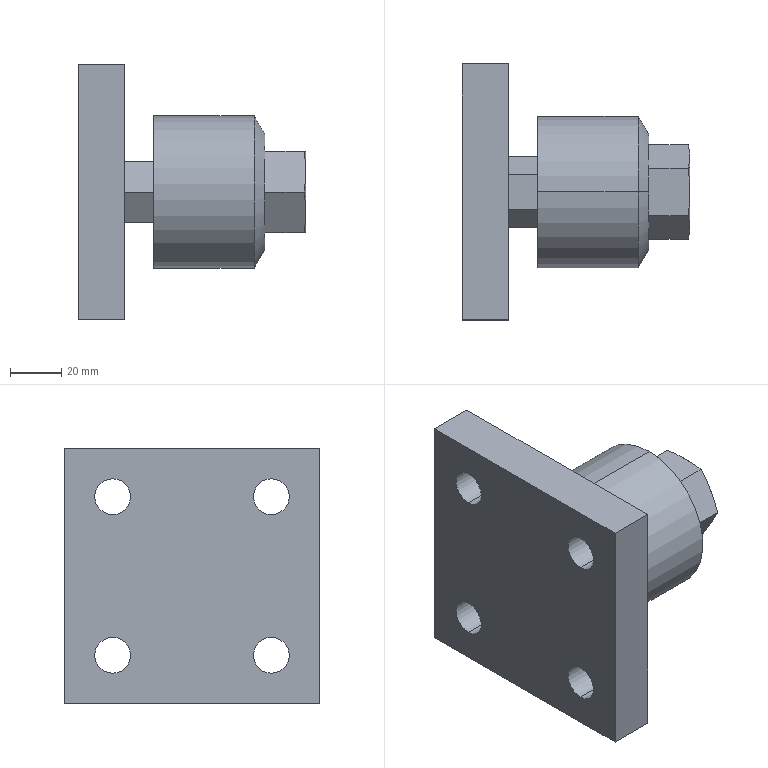Part | SolidWorks | features BaseBody 2 | 2 solids | 46 faces | box 89 x 100 x 100 mm | volume 301909 mm3 | plane 22 | cylinder 12 | cone 12 | commonest cylinder face diameters 14 x8 18.376 x2 59.5 x2
STEP:
#1=CARTESIAN_POINT('',(-59.5,0.,-29.75));
#2=VERTEX_POINT('',#1);
#3=CARTESIAN_POINT('',(-59.5,0.,29.75));
#4=VERTEX_POINT('',#3);
#5=CARTESIAN_POINT('',(-59.5,0.,0.));
#6=DIRECTION('',(1.,0.,0.));
#7=DIRECTION('',(0.,0.,-1.));
#8=AXIS2_PLACEMENT_3D('',#5,#6,#7);
#9=CIRCLE('',#8,29.75);
#10=EDGE_CURVE('',#2,#4,#9,.T.);
#11=ORIENTED_EDGE('',*,*,#10,.T.);
#12=CARTESIAN_POINT('',(-20.186,0.,29.75));
#13=VERTEX_POINT('',#12);
#14=CARTESIAN_POINT('',(-39.843,0.,29.75));
#15=DIRECTION('',(1.,0.,0.));
#16=VECTOR('',#15,1000.);
#17=LINE('',#14,#16);
#18=EDGE_CURVE('',#4,#13,#17,.T.);
#19=ORIENTED_EDGE('',*,*,#18,.T.);
#20=CARTESIAN_POINT('',(-20.186,0.,-29.75));
#21=VERTEX_POINT('',#20);
#22=CARTESIAN_POINT('',(-20.186,0.,0.));
#23=DIRECTION('',(-1.,0.,0.));
#24=DIRECTION('',(0.,0.,-1.));
#25=AXIS2_PLACEMENT_3D('',#22,#23,#24);
#26=CIRCLE('',#25,29.75);
#27=EDGE_CURVE('',#13,#21,#26,.T.);
#28=ORIENTED_EDGE('',*,*,#27,.T.);
#29=CARTESIAN_POINT('',(-39.843,0.,-29.75));
#30=DIRECTION('',(1.,0.,0.));
#31=VECTOR('',#30,1000.);
#32=LINE('',#29,#31);
#33=EDGE_CURVE('',#2,#21,#32,.T.);
#34=ORIENTED_EDGE('',*,*,#33,.F.);
#35=EDGE_LOOP('',(#11,#19,#28,#34));
#36=FACE_OUTER_BOUND('',#35,.T.);
#37=CARTESIAN_POINT('',(-39.843,0.,0.));
#38=DIRECTION('',(1.,0.,0.));
#39=DIRECTION('',(0.,0.,-1.));
#40=AXIS2_PLACEMENT_3D('',#37,#38,#39);
#41=CYLINDRICAL_SURFACE('',#40,29.75);
#42=ADVANCED_FACE('',(#36),#41,.T.);
#43=CARTESIAN_POINT('',(-16.,0.,22.5));
#44=VERTEX_POINT('',#43);
#45=CARTESIAN_POINT('',(-16.,0.,-22.5));
#46=VERTEX_POINT('',#45);
#47=CARTESIAN_POINT('',(-16.,0.,0.));
#48=DIRECTION('',(-1.,0.,0.));
#49=DIRECTION('',(0.,0.,1.));
#50=AXIS2_PLACEMENT_3D('',#47,#48,#49);
#51=CIRCLE('',#50,22.5);
#52=EDGE_CURVE('',#44,#46,#51,.T.);
#53=ORIENTED_EDGE('',*,*,#52,.T.);
#54=CARTESIAN_POINT('',(-20.186,0.,-29.75));
#55=DIRECTION('',(-0.5,0.,-0.866));
#56=VECTOR('',#55,1000.);
#57=LINE('',#54,#56);
#58=EDGE_CURVE('',#46,#21,#57,.T.);
#59=ORIENTED_EDGE('',*,*,#58,.T.);
#60=ORIENTED_EDGE('',*,*,#27,.F.);
#61=CARTESIAN_POINT('',(-20.186,0.,29.75));
#62=DIRECTION('',(-0.5,0.,0.866));
#63=VECTOR('',#62,1000.);
#64=LINE('',#61,#63);
#65=EDGE_CURVE('',#44,#13,#64,.T.);
#66=ORIENTED_EDGE('',*,*,#65,.F.);
#67=EDGE_LOOP('',(#53,#59,#60,#66));
#68=FACE_OUTER_BOUND('',#67,.T.);
#69=CARTESIAN_POINT('',(-20.186,0.,0.));
#70=DIRECTION('',(-1.,0.,0.));
#71=DIRECTION('',(0.,0.,1.));
#72=AXIS2_PLACEMENT_3D('',#69,#70,#71);
#73=CONICAL_SURFACE('',#72,29.75,1.047);
#74=ADVANCED_FACE('',(#68),#73,.T.);
#75=CARTESIAN_POINT('',(-0.812,0.,9.188));
#76=VERTEX_POINT('',#75);
#77=CARTESIAN_POINT('',(-0.812,0.,-9.188));
#78=VERTEX_POINT('',#77);
#79=CARTESIAN_POINT('',(-0.812,0.,0.));
#80=DIRECTION('',(1.,0.,0.));
#81=DIRECTION('',(0.,0.,-1.));
#82=AXIS2_PLACEMENT_3D('',#79,#80,#81);
#83=CIRCLE('',#82,9.188);
#84=EDGE_CURVE('',#76,#78,#83,.T.);
#85=ORIENTED_EDGE('',*,*,#84,.F.);
#86=CARTESIAN_POINT('',(0.,0.,10.));
#87=VERTEX_POINT('',#86);
#88=CARTESIAN_POINT('',(0.,0.,10.));
#89=DIRECTION('',(0.7071,0.,0.7071));
#90=VECTOR('',#89,1000.);
#91=LINE('',#88,#90);
#92=EDGE_CURVE('',#76,#87,#91,.T.);
#93=ORIENTED_EDGE('',*,*,#92,.T.);
#94=CARTESIAN_POINT('',(0.,0.,-10.));
#95=VERTEX_POINT('',#94);
#96=CARTESIAN_POINT('',(0.,0.,0.));
#97=DIRECTION('',(-1.,0.,0.));
#98=DIRECTION('',(0.,0.,-1.));
#99=AXIS2_PLACEMENT_3D('',#96,#97,#98);
#100=CIRCLE('',#99,10.);
#101=EDGE_CURVE('',#95,#87,#100,.T.);
#102=ORIENTED_EDGE('',*,*,#101,.F.);
#103=CARTESIAN_POINT('',(0.,0.,-10.));
#104=DIRECTION('',(0.7071,0.,-0.7071));
#105=VECTOR('',#104,1000.);
#106=LINE('',#103,#105);
#107=EDGE_CURVE('',#78,#95,#106,.T.);
#108=ORIENTED_EDGE('',*,*,#107,.F.);
#109=EDGE_LOOP('',(#85,#93,#102,#108));
#110=FACE_OUTER_BOUND('',#109,.T.);
#111=CARTESIAN_POINT('',(0.,0.,0.));
#112=DIRECTION('',(1.,0.,0.));
#113=DIRECTION('',(0.,0.,-1.));
#114=AXIS2_PLACEMENT_3D('',#111,#112,#113);
#115=CONICAL_SURFACE('',#114,10.,0.7854);
#116=ADVANCED_FACE('',(#110),#115,.F.);
#117=CARTESIAN_POINT('',(-18.,0.,9.188));
#118=VERTEX_POINT('',#117);
#119=CARTESIAN_POINT('',(-18.,0.,-9.188));
#120=VERTEX_POINT('',#119);
#121=CARTESIAN_POINT('',(-18.,0.,0.));
#122=DIRECTION('',(1.,0.,0.));
#123=DIRECTION('',(0.,0.,-1.));
#124=AXIS2_PLACEMENT_3D('',#121,#122,#123);
#125=CIRCLE('',#124,9.188);
#126=EDGE_CURVE('',#118,#120,#125,.T.);
#127=ORIENTED_EDGE('',*,*,#126,.F.);
#128=CARTESIAN_POINT('',(-9.406,0.,9.188));
#129=DIRECTION('',(1.,0.,0.));
#130=VECTOR('',#129,1000.);
#131=LINE('',#128,#130);
#132=EDGE_CURVE('',#118,#76,#131,.T.);
#133=ORIENTED_EDGE('',*,*,#132,.T.);
#134=ORIENTED_EDGE('',*,*,#84,.T.);
#135=CARTESIAN_POINT('',(-9.406,0.,-9.188));
#136=DIRECTION('',(1.,0.,0.));
#137=VECTOR('',#136,1000.);
#138=LINE('',#135,#137);
#139=EDGE_CURVE('',#120,#78,#138,.T.);
#140=ORIENTED_EDGE('',*,*,#139,.F.);
#141=EDGE_LOOP('',(#127,#133,#134,#140));
#142=FACE_OUTER_BOUND('',#141,.T.);
#143=CARTESIAN_POINT('',(-9.406,0.,0.));
#144=DIRECTION('',(1.,0.,0.));
#145=DIRECTION('',(0.,0.,-1.));
#146=AXIS2_PLACEMENT_3D('',#143,#144,#145);
#147=CYLINDRICAL_SURFACE('',#146,9.188);
#148=ADVANCED_FACE('',(#142),#147,.F.);
#149=CARTESIAN_POINT('',(-23.305,0.,0.));
#150=VERTEX_POINT('',#149);
#151=CARTESIAN_POINT('',(-18.,0.,-9.188));
#152=DIRECTION('',(0.5,0.,-0.866));
#153=VECTOR('',#152,1000.);
#154=LINE('',#151,#153);
#155=EDGE_CURVE('',#150,#120,#154,.T.);
#156=ORIENTED_EDGE('',*,*,#155,.F.);
#157=CARTESIAN_POINT('',(-18.,0.,9.188));
#158=DIRECTION('',(0.5,0.,0.866));
#159=VECTOR('',#158,1000.);
#160=LINE('',#157,#159);
#161=EDGE_CURVE('',#150,#118,#160,.T.);
#162=ORIENTED_EDGE('',*,*,#161,.T.);
#163=ORIENTED_EDGE('',*,*,#126,.T.);
#164=EDGE_LOOP('',(#156,#162,#163));
#165=FACE_OUTER_BOUND('',#164,.T.);
#166=CARTESIAN_POINT('',(-18.,0.,0.));
#167=DIRECTION('',(1.,0.,0.));
#168=DIRECTION('',(0.,0.,-1.));
#169=AXIS2_PLACEMENT_3D('',#166,#167,#168);
#170=CONICAL_SURFACE('',#169,9.188,1.047);
#171=ADVANCED_FACE('',(#165),#170,.F.);
#172=ORIENTED_EDGE('',*,*,#18,.F.);
#173=CARTESIAN_POINT('',(-59.5,0.,0.));
#174=DIRECTION('',(1.,0.,0.));
#175=DIRECTION('',(0.,0.,-1.));
#176=AXIS2_PLACEMENT_3D('',#173,#174,#175);
#177=CIRCLE('',#176,29.75);
#178=EDGE_CURVE('',#4,#2,#177,.T.);
#179=ORIENTED_EDGE('',*,*,#178,.T.);
#180=ORIENTED_EDGE('',*,*,#33,.T.);
#181=CARTESIAN_POINT('',(-20.186,0.,0.));
#182=DIRECTION('',(-1.,0.,0.));
#183=DIRECTION('',(0.,0.,-1.));
#184=AXIS2_PLACEMENT_3D('',#181,#182,#183);
#185=CIRCLE('',#184,29.75);
#186=EDGE_CURVE('',#21,#13,#185,.T.);
#187=ORIENTED_EDGE('',*,*,#186,.T.);
#188=EDGE_LOOP('',(#172,#179,#180,#187));
#189=FACE_OUTER_BOUND('',#188,.T.);
#190=CARTESIAN_POINT('',(-39.843,0.,0.));
#191=DIRECTION('',(1.,0.,0.));
#192=DIRECTION('',(0.,0.,-1.));
#193=AXIS2_PLACEMENT_3D('',#190,#191,#192);
#194=CYLINDRICAL_SURFACE('',#193,29.75);
#195=ADVANCED_FACE('',(#189),#194,.T.);
#196=ORIENTED_EDGE('',*,*,#58,.F.);
#197=CARTESIAN_POINT('',(-16.,0.,0.));
#198=DIRECTION('',(-1.,0.,0.));
#199=DIRECTION('',(0.,0.,1.));
#200=AXIS2_PLACEMENT_3D('',#197,#198,#199);
#201=CIRCLE('',#200,22.5);
#202=EDGE_CURVE('',#46,#44,#201,.T.);
#203=ORIENTED_EDGE('',*,*,#202,.T.);
#204=ORIENTED_EDGE('',*,*,#65,.T.);
#205=ORIENTED_EDGE('',*,*,#186,.F.);
#206=EDGE_LOOP('',(#196,#203,#204,#205));
#207=FACE_OUTER_BOUND('',#206,.T.);
#208=CARTESIAN_POINT('',(-20.186,0.,0.));
#209=DIRECTION('',(-1.,0.,0.));
#210=DIRECTION('',(0.,0.,1.));
#211=AXIS2_PLACEMENT_3D('',#208,#209,#210);
#212=CONICAL_SURFACE('',#211,29.75,1.047);
#213=ADVANCED_FACE('',(#207),#212,.T.);
#214=CARTESIAN_POINT('',(-59.5,-13.856,0.));
#215=VERTEX_POINT('',#214);
#216=CARTESIAN_POINT('',(-59.5,-6.928,-12.));
#217=VERTEX_POINT('',#216);
#218=CARTESIAN_POINT('',(-59.5,-13.856,0.));
#219=DIRECTION('',(0.,0.5,-0.866));
#220=VECTOR('',#219,1000.);
#221=LINE('',#218,#220);
#222=EDGE_CURVE('',#215,#217,#221,.T.);
#223=ORIENTED_EDGE('',*,*,#222,.T.);
#224=CARTESIAN_POINT('',(-59.5,6.928,-12.));
#225=VERTEX_POINT('',#224);
#226=CARTESIAN_POINT('',(-59.5,22.075,-12.));
#227=DIRECTION('',(0.,1.,0.));
#228=VECTOR('',#227,1000.);
#229=LINE('',#226,#228);
#230=EDGE_CURVE('',#217,#225,#229,.T.);
#231=ORIENTED_EDGE('',*,*,#230,.T.);
#232=CARTESIAN_POINT('',(-59.5,13.856,0.));
#233=VERTEX_POINT('',#232);
#234=CARTESIAN_POINT('',(-59.5,6.928,-12.));
#235=DIRECTION('',(0.,0.5,0.866));
#236=VECTOR('',#235,1000.);
#237=LINE('',#234,#236);
#238=EDGE_CURVE('',#225,#233,#237,.T.);
#239=ORIENTED_EDGE('',*,*,#238,.T.);
#240=CARTESIAN_POINT('',(-59.5,6.928,12.));
#241=VERTEX_POINT('',#240);
#242=CARTESIAN_POINT('',(-59.5,13.856,0.));
#243=DIRECTION('',(0.,-0.5,0.866));
#244=VECTOR('',#243,1000.);
#245=LINE('',#242,#244);
#246=EDGE_CURVE('',#233,#241,#245,.T.);
#247=ORIENTED_EDGE('',*,*,#246,.T.);
#248=CARTESIAN_POINT('',(-59.5,-6.928,12.));
#249=VERTEX_POINT('',#248);
#250=CARTESIAN_POINT('',(-59.5,22.075,12.));
#251=DIRECTION('',(0.,-1.,0.));
#252=VECTOR('',#251,1000.);
#253=LINE('',#250,#252);
#254=EDGE_CURVE('',#241,#249,#253,.T.);
#255=ORIENTED_EDGE('',*,*,#254,.T.);
#256=CARTESIAN_POINT('',(-59.5,-6.928,12.));
#257=DIRECTION('',(0.,-0.5,-0.866));
#258=VECTOR('',#257,1000.);
#259=LINE('',#256,#258);
#260=EDGE_CURVE('',#249,#215,#259,.T.);
#261=ORIENTED_EDGE('',*,*,#260,.T.);
#262=EDGE_LOOP('',(#223,#231,#239,#247,#255,#261));
#263=FACE_BOUND('',#262,.T.);
#264=ORIENTED_EDGE('',*,*,#10,.F.);
#265=ORIENTED_EDGE('',*,*,#178,.F.);
#266=EDGE_LOOP('',(#264,#265));
#267=FACE_OUTER_BOUND('',#266,.T.);
#268=CARTESIAN_POINT('',(-59.5,22.075,0.));
#269=DIRECTION('',(-1.,0.,0.));
#270=DIRECTION('',(0.,0.,1.));
#271=AXIS2_PLACEMENT_3D('',#268,#269,#270);
#272=PLANE('',#271);
#273=ADVANCED_FACE('',(#263,#267),#272,.T.);
#274=CARTESIAN_POINT('',(-16.,-9.238,16.));
#275=VERTEX_POINT('',#274);
#276=CARTESIAN_POINT('',(-16.,9.238,16.));
#277=VERTEX_POINT('',#276);
#278=CARTESIAN_POINT('',(-16.,20.488,16.));
#279=DIRECTION('',(0.,1.,0.));
#280=VECTOR('',#279,1000.);
#281=LINE('',#278,#280);
#282=EDGE_CURVE('',#275,#277,#281,.T.);
#283=ORIENTED_EDGE('',*,*,#282,.T.);
#284=CARTESIAN_POINT('',(-16.,18.475,0.));
#285=VERTEX_POINT('',#284);
#286=CARTESIAN_POINT('',(-16.,9.238,16.));
#287=DIRECTION('',(0.,0.5,-0.866));
#288=VECTOR('',#287,1000.);
#289=LINE('',#286,#288);
#290=EDGE_CURVE('',#277,#285,#289,.T.);
#291=ORIENTED_EDGE('',*,*,#290,.T.);
#292=CARTESIAN_POINT('',(-16.,9.238,-16.));
#293=VERTEX_POINT('',#292);
#294=CARTESIAN_POINT('',(-16.,18.475,0.));
#295=DIRECTION('',(0.,-0.5,-0.866));
#296=VECTOR('',#295,1000.);
#297=LINE('',#294,#296);
#298=EDGE_CURVE('',#285,#293,#297,.T.);
#299=ORIENTED_EDGE('',*,*,#298,.T.);
#300=CARTESIAN_POINT('',(-16.,-9.238,-16.));
#301=VERTEX_POINT('',#300);
#302=CARTESIAN_POINT('',(-16.,20.488,-16.));
#303=DIRECTION('',(0.,-1.,0.));
#304=VECTOR('',#303,1000.);
#305=LINE('',#302,#304);
#306=EDGE_CURVE('',#293,#301,#305,.T.);
#307=ORIENTED_EDGE('',*,*,#306,.T.);
#308=CARTESIAN_POINT('',(-16.,-18.475,0.));
#309=VERTEX_POINT('',#308);
#310=CARTESIAN_POINT('',(-16.,-9.238,-16.));
#311=DIRECTION('',(0.,-0.5,0.866));
#312=VECTOR('',#311,1000.);
#313=LINE('',#310,#312);
#314=EDGE_CURVE('',#301,#309,#313,.T.);
#315=ORIENTED_EDGE('',*,*,#314,.T.);
#316=CARTESIAN_POINT('',(-16.,-18.475,0.));
#317=DIRECTION('',(0.,0.5,0.866));
#318=VECTOR('',#317,1000.);
#319=LINE('',#316,#318);
#320=EDGE_CURVE('',#309,#275,#319,.T.);
#321=ORIENTED_EDGE('',*,*,#320,.T.);
#322=EDGE_LOOP('',(#283,#291,#299,#307,#315,#321));
#323=FACE_BOUND('',#322,.T.);
#324=ORIENTED_EDGE('',*,*,#52,.F.);
#325=ORIENTED_EDGE('',*,*,#202,.F.);
#326=EDGE_LOOP('',(#324,#325));
#327=FACE_OUTER_BOUND('',#326,.T.);
#328=CARTESIAN_POINT('',(-16.,20.488,0.));
#329=DIRECTION('',(1.,0.,0.));
#330=DIRECTION('',(0.,0.,-1.));
#331=AXIS2_PLACEMENT_3D('',#328,#329,#330);
#332=PLANE('',#331);
#333=ADVANCED_FACE('',(#323,#327),#332,.T.);
#334=CARTESIAN_POINT('',(-71.,6.928,-12.));
#335=VERTEX_POINT('',#334);
#336=CARTESIAN_POINT('',(-71.,-6.928,-12.));
#337=VERTEX_POINT('',#336);
#338=CARTESIAN_POINT('',(-71.,-6.928,-12.));
#339=DIRECTION('',(0.,-1.,0.));
#340=VECTOR('',#339,1000.);
#341=LINE('',#338,#340);
#342=EDGE_CURVE('',#335,#337,#341,.T.);
#343=ORIENTED_EDGE('',*,*,#342,.F.);
#344=CARTESIAN_POINT('',(-71.,6.928,-12.));
#345=DIRECTION('',(-1.,0.,0.));
#346=VECTOR('',#345,1000.);
#347=LINE('',#344,#346);
#348=EDGE_CURVE('',#225,#335,#347,.T.);
#349=ORIENTED_EDGE('',*,*,#348,.F.);
#350=ORIENTED_EDGE('',*,*,#230,.F.);
#351=CARTESIAN_POINT('',(-71.,-6.928,-12.));
#352=DIRECTION('',(1.,0.,0.));
#353=VECTOR('',#352,1000.);
#354=LINE('',#351,#353);
#355=EDGE_CURVE('',#337,#217,#354,.T.);
#356=ORIENTED_EDGE('',*,*,#355,.F.);
#357=EDGE_LOOP('',(#343,#349,#350,#356));
#358=FACE_OUTER_BOUND('',#357,.T.);
#359=CARTESIAN_POINT('',(-71.,-6.928,-12.));
#360=DIRECTION('',(0.,0.,1.));
#361=DIRECTION('',(1.,0.,0.));
#362=AXIS2_PLACEMENT_3D('',#359,#360,#361);
#363=PLANE('',#362);
#364=ADVANCED_FACE('',(#358),#363,.F.);
#365=CARTESIAN_POINT('',(-71.,-13.856,0.));
#366=VERTEX_POINT('',#365);
#367=CARTESIAN_POINT('',(-71.,-13.856,0.));
#368=DIRECTION('',(0.,-0.5,0.866));
#369=VECTOR('',#368,1000.);
#370=LINE('',#367,#369);
#371=EDGE_CURVE('',#337,#366,#370,.T.);
#372=ORIENTED_EDGE('',*,*,#371,.F.);
#373=ORIENTED_EDGE('',*,*,#355,.T.);
#374=ORIENTED_EDGE('',*,*,#222,.F.);
#375=CARTESIAN_POINT('',(-71.,-13.856,0.));
#376=DIRECTION('',(1.,0.,0.));
#377=VECTOR('',#376,1000.);
#378=LINE('',#375,#377);
#379=EDGE_CURVE('',#366,#215,#378,.T.);
#380=ORIENTED_EDGE('',*,*,#379,.F.);
#381=EDGE_LOOP('',(#372,#373,#374,#380));
#382=FACE_OUTER_BOUND('',#381,.T.);
#383=CARTESIAN_POINT('',(-71.,-13.856,0.));
#384=DIRECTION('',(0.,0.866,0.5));
#385=DIRECTION('',(0.,-0.5,0.866));
#386=AXIS2_PLACEMENT_3D('',#383,#384,#385);
#387=PLANE('',#386);
#388=ADVANCED_FACE('',(#382),#387,.F.);
#389=CARTESIAN_POINT('',(-71.,-6.928,12.));
#390=VERTEX_POINT('',#389);
#391=CARTESIAN_POINT('',(-71.,-6.928,12.));
#392=DIRECTION('',(0.,0.5,0.866));
#393=VECTOR('',#392,1000.);
#394=LINE('',#391,#393);
#395=EDGE_CURVE('',#366,#390,#394,.T.);
#396=ORIENTED_EDGE('',*,*,#395,.F.);
#397=ORIENTED_EDGE('',*,*,#379,.T.);
#398=ORIENTED_EDGE('',*,*,#260,.F.);
#399=CARTESIAN_POINT('',(-71.,-6.928,12.));
#400=DIRECTION('',(1.,0.,0.));
#401=VECTOR('',#400,1000.);
#402=LINE('',#399,#401);
#403=EDGE_CURVE('',#390,#249,#402,.T.);
#404=ORIENTED_EDGE('',*,*,#403,.F.);
#405=EDGE_LOOP('',(#396,#397,#398,#404));
#406=FACE_OUTER_BOUND('',#405,.T.);
#407=CARTESIAN_POINT('',(-71.,-6.928,12.));
#408=DIRECTION('',(0.,0.866,-0.5));
#409=DIRECTION('',(0.,0.5,0.866));
#410=AXIS2_PLACEMENT_3D('',#407,#408,#409);
#411=PLANE('',#410);
#412=ADVANCED_FACE('',(#406),#411,.F.);
#413=CARTESIAN_POINT('',(-71.,6.928,12.));
#414=VERTEX_POINT('',#413);
#415=CARTESIAN_POINT('',(-71.,6.928,12.));
#416=DIRECTION('',(0.,1.,0.));
#417=VECTOR('',#416,1000.);
#418=LINE('',#415,#417);
#419=EDGE_CURVE('',#390,#414,#418,.T.);
#420=ORIENTED_EDGE('',*,*,#419,.F.);
#421=ORIENTED_EDGE('',*,*,#403,.T.);
#422=ORIENTED_EDGE('',*,*,#254,.F.);
#423=CARTESIAN_POINT('',(-71.,6.928,12.));
#424=DIRECTION('',(1.,0.,0.));
#425=VECTOR('',#424,1000.);
#426=LINE('',#423,#425);
#427=EDGE_CURVE('',#414,#241,#426,.T.);
#428=ORIENTED_EDGE('',*,*,#427,.F.);
#429=EDGE_LOOP('',(#420,#421,#422,#428));
#430=FACE_OUTER_BOUND('',#429,.T.);
#431=CARTESIAN_POINT('',(-71.,6.928,12.));
#432=DIRECTION('',(0.,0.,-1.));
#433=DIRECTION('',(-1.,0.,0.));
#434=AXIS2_PLACEMENT_3D('',#431,#432,#433);
#435=PLANE('',#434);
#436=ADVANCED_FACE('',(#430),#435,.F.);
#437=CARTESIAN_POINT('',(-71.,13.856,0.));
#438=VERTEX_POINT('',#437);
#439=CARTESIAN_POINT('',(-71.,13.856,0.));
#440=DIRECTION('',(0.,0.5,-0.866));
#441=VECTOR('',#440,1000.);
#442=LINE('',#439,#441);
#443=EDGE_CURVE('',#414,#438,#442,.T.);
#444=ORIENTED_EDGE('',*,*,#443,.F.);
#445=ORIENTED_EDGE('',*,*,#427,.T.);
#446=ORIENTED_EDGE('',*,*,#246,.F.);
#447=CARTESIAN_POINT('',(-71.,13.856,0.));
#448=DIRECTION('',(1.,0.,0.));
#449=VECTOR('',#448,1000.);
#450=LINE('',#447,#449);
#451=EDGE_CURVE('',#438,#233,#450,.T.);
#452=ORIENTED_EDGE('',*,*,#451,.F.);
#453=EDGE_LOOP('',(#444,#445,#446,#452));
#454=FACE_OUTER_BOUND('',#453,.T.);
#455=CARTESIAN_POINT('',(-71.,13.856,0.));
#456=DIRECTION('',(0.,-0.866,-0.5));
#457=DIRECTION('',(0.,0.5,-0.866));
#458=AXIS2_PLACEMENT_3D('',#455,#456,#457);
#459=PLANE('',#458);
#460=ADVANCED_FACE('',(#454),#459,.F.);
#461=CARTESIAN_POINT('',(-71.,6.928,-12.));
#462=DIRECTION('',(0.,-0.5,-0.866));
#463=VECTOR('',#462,1000.);
#464=LINE('',#461,#463);
#465=EDGE_CURVE('',#438,#335,#464,.T.);
#466=ORIENTED_EDGE('',*,*,#465,.F.);
#467=ORIENTED_EDGE('',*,*,#451,.T.);
#468=ORIENTED_EDGE('',*,*,#238,.F.);
#469=ORIENTED_EDGE('',*,*,#348,.T.);
#470=EDGE_LOOP('',(#466,#467,#468,#469));
#471=FACE_OUTER_BOUND('',#470,.T.);
#472=CARTESIAN_POINT('',(-71.,6.928,-12.));
#473=DIRECTION('',(0.,-0.866,0.5));
#474=DIRECTION('',(0.,-0.5,-0.866));
#475=AXIS2_PLACEMENT_3D('',#472,#473,#474);
#476=PLANE('',#475);
#477=ADVANCED_FACE('',(#471),#476,.F.);
#478=ORIENTED_EDGE('',*,*,#290,.F.);
#479=CARTESIAN_POINT('',(-0.6632,9.238,16.));
#480=VERTEX_POINT('',#479);
#481=CARTESIAN_POINT('',(0.,9.238,16.));
#482=DIRECTION('',(-1.,0.,0.));
#483=VECTOR('',#482,1000.);
#484=LINE('',#481,#483);
#485=EDGE_CURVE('',#480,#277,#484,.T.);
#486=ORIENTED_EDGE('',*,*,#485,.F.);
#487=CARTESIAN_POINT('',(0.,13.856,8.));
#488=VERTEX_POINT('',#487);
#489=CARTESIAN_POINT('',(0.,13.856,8.));
#490=CARTESIAN_POINT('',(0.,13.083,9.34));
#491=CARTESIAN_POINT('',(-0.06124,12.311,10.677));
#492=CARTESIAN_POINT('',(-0.2905,10.772,13.343));
#493=CARTESIAN_POINT('',(-0.4579,10.004,14.673));
#494=CARTESIAN_POINT('',(-0.6632,9.238,16.));
#495=B_SPLINE_CURVE_WITH_KNOTS('',3,(#489,#490,#491,#492,#493,#494),.UNSPECIFIED.,.F.,.F.,(4,2,4),(0.,0.004631,0.009261),.UNSPECIFIED.);
#496=EDGE_CURVE('',#488,#480,#495,.T.);
#497=ORIENTED_EDGE('',*,*,#496,.F.);
#498=CARTESIAN_POINT('',(-0.6632,18.475,0.));
#499=VERTEX_POINT('',#498);
#500=CARTESIAN_POINT('',(-0.6632,18.475,0.));
#501=CARTESIAN_POINT('',(-0.4579,17.709,1.327));
#502=CARTESIAN_POINT('',(-0.2905,16.941,2.657));
#503=CARTESIAN_POINT('',(-0.06124,15.402,5.323));
#504=CARTESIAN_POINT('',(0.,14.63,6.66));
#505=CARTESIAN_POINT('',(0.,13.856,8.));
#506=B_SPLINE_CURVE_WITH_KNOTS('',3,(#500,#501,#502,#503,#504,#505),.UNSPECIFIED.,.F.,.F.,(4,2,4),(0.,0.004631,0.009261),.UNSPECIFIED.);
#507=EDGE_CURVE('',#499,#488,#506,.T.);
#508=ORIENTED_EDGE('',*,*,#507,.F.);
#509=CARTESIAN_POINT('',(0.,18.475,0.));
#510=DIRECTION('',(1.,0.,0.));
#511=VECTOR('',#510,1000.);
#512=LINE('',#509,#511);
#513=EDGE_CURVE('',#285,#499,#512,.T.);
#514=ORIENTED_EDGE('',*,*,#513,.F.);
#515=EDGE_LOOP('',(#478,#486,#497,#508,#514));
#516=FACE_OUTER_BOUND('',#515,.T.);
#517=CARTESIAN_POINT('',(0.,9.238,16.));
#518=DIRECTION('',(0.,-0.866,-0.5));
#519=DIRECTION('',(0.,0.5,-0.866));
#520=AXIS2_PLACEMENT_3D('',#517,#518,#519);
#521=PLANE('',#520);
#522=ADVANCED_FACE('',(#516),#521,.F.);
#523=ORIENTED_EDGE('',*,*,#485,.T.);
#524=ORIENTED_EDGE('',*,*,#282,.F.);
#525=CARTESIAN_POINT('',(-0.6632,-9.238,16.));
#526=VERTEX_POINT('',#525);
#527=CARTESIAN_POINT('',(0.,-9.238,16.));
#528=DIRECTION('',(-1.,0.,0.));
#529=VECTOR('',#528,1000.);
#530=LINE('',#527,#529);
#531=EDGE_CURVE('',#526,#275,#530,.T.);
#532=ORIENTED_EDGE('',*,*,#531,.F.);
#533=CARTESIAN_POINT('',(0.,0.,16.));
#534=VERTEX_POINT('',#533);
#535=CARTESIAN_POINT('',(0.,0.,16.));
#536=CARTESIAN_POINT('',(0.,-1.548,16.));
#537=CARTESIAN_POINT('',(-0.06124,-3.091,16.));
#538=CARTESIAN_POINT('',(-0.2905,-6.169,16.));
#539=CARTESIAN_POINT('',(-0.4579,-7.705,16.));
#540=CARTESIAN_POINT('',(-0.6632,-9.238,16.));
#541=B_SPLINE_CURVE_WITH_KNOTS('',3,(#535,#536,#537,#538,#539,#540),.UNSPECIFIED.,.F.,.F.,(4,2,4),(0.,0.004631,0.009261),.UNSPECIFIED.);
#542=EDGE_CURVE('',#534,#526,#541,.T.);
#543=ORIENTED_EDGE('',*,*,#542,.F.);
#544=CARTESIAN_POINT('',(-0.6632,9.238,16.));
#545=CARTESIAN_POINT('',(-0.4579,7.705,16.));
#546=CARTESIAN_POINT('',(-0.2905,6.169,16.));
#547=CARTESIAN_POINT('',(-0.06124,3.091,16.));
#548=CARTESIAN_POINT('',(0.,1.548,16.));
#549=CARTESIAN_POINT('',(0.,0.,16.));
#550=B_SPLINE_CURVE_WITH_KNOTS('',3,(#544,#545,#546,#547,#548,#549),.UNSPECIFIED.,.F.,.F.,(4,2,4),(0.,0.004631,0.009261),.UNSPECIFIED.);
#551=EDGE_CURVE('',#480,#534,#550,.T.);
#552=ORIENTED_EDGE('',*,*,#551,.F.);
#553=EDGE_LOOP('',(#523,#524,#532,#543,#552));
#554=FACE_OUTER_BOUND('',#553,.T.);
#555=CARTESIAN_POINT('',(0.,-9.238,16.));
#556=DIRECTION('',(0.,0.,-1.));
#557=DIRECTION('',(-1.,0.,0.));
#558=AXIS2_PLACEMENT_3D('',#555,#556,#557);
#559=PLANE('',#558);
#560=ADVANCED_FACE('',(#554),#559,.F.);
#561=ORIENTED_EDGE('',*,*,#531,.T.);
#562=ORIENTED_EDGE('',*,*,#320,.F.);
#563=CARTESIAN_POINT('',(-0.6632,-18.475,0.));
#564=VERTEX_POINT('',#563);
#565=CARTESIAN_POINT('',(0.,-18.475,0.));
#566=DIRECTION('',(-1.,0.,0.));
#567=VECTOR('',#566,1000.);
#568=LINE('',#565,#567);
#569=EDGE_CURVE('',#564,#309,#568,.T.);
#570=ORIENTED_EDGE('',*,*,#569,.F.);
#571=CARTESIAN_POINT('',(0.,-13.856,8.));
#572=VERTEX_POINT('',#571);
#573=CARTESIAN_POINT('',(0.,-13.856,8.));
#574=CARTESIAN_POINT('',(0.,-14.63,6.66));
#575=CARTESIAN_POINT('',(-0.06124,-15.402,5.323));
#576=CARTESIAN_POINT('',(-0.2905,-16.941,2.657));
#577=CARTESIAN_POINT('',(-0.4579,-17.709,1.327));
#578=CARTESIAN_POINT('',(-0.6632,-18.475,0.));
#579=B_SPLINE_CURVE_WITH_KNOTS('',3,(#573,#574,#575,#576,#577,#578),.UNSPECIFIED.,.F.,.F.,(4,2,4),(0.,0.004631,0.009261),.UNSPECIFIED.);
#580=EDGE_CURVE('',#572,#564,#579,.T.);
#581=ORIENTED_EDGE('',*,*,#580,.F.);
#582=CARTESIAN_POINT('',(-0.6632,-9.238,16.));
#583=CARTESIAN_POINT('',(-0.4579,-10.004,14.673));
#584=CARTESIAN_POINT('',(-0.2905,-10.772,13.343));
#585=CARTESIAN_POINT('',(-0.06124,-12.311,10.677));
#586=CARTESIAN_POINT('',(0.,-13.083,9.34));
#587=CARTESIAN_POINT('',(0.,-13.856,8.));
#588=B_SPLINE_CURVE_WITH_KNOTS('',3,(#582,#583,#584,#585,#586,#587),.UNSPECIFIED.,.F.,.F.,(4,2,4),(0.,0.004631,0.009261),.UNSPECIFIED.);
#589=EDGE_CURVE('',#526,#572,#588,.T.);
#590=ORIENTED_EDGE('',*,*,#589,.F.);
#591=EDGE_LOOP('',(#561,#562,#570,#581,#590));
#592=FACE_OUTER_BOUND('',#591,.T.);
#593=CARTESIAN_POINT('',(0.,-18.475,0.));
#594=DIRECTION('',(0.,0.866,-0.5));
#595=DIRECTION('',(0.,0.5,0.866));
#596=AXIS2_PLACEMENT_3D('',#593,#594,#595);
#597=PLANE('',#596);
#598=ADVANCED_FACE('',(#592),#597,.F.);
#599=ORIENTED_EDGE('',*,*,#569,.T.);
#600=ORIENTED_EDGE('',*,*,#314,.F.);
#601=CARTESIAN_POINT('',(-0.6632,-9.238,-16.));
#602=VERTEX_POINT('',#601);
#603=CARTESIAN_POINT('',(0.,-9.238,-16.));
#604=DIRECTION('',(-1.,0.,0.));
#605=VECTOR('',#604,1000.);
#606=LINE('',#603,#605);
#607=EDGE_CURVE('',#602,#301,#606,.T.);
#608=ORIENTED_EDGE('',*,*,#607,.F.);
#609=CARTESIAN_POINT('',(0.,-13.856,-8.));
#610=VERTEX_POINT('',#609);
#611=CARTESIAN_POINT('',(0.,-13.856,-8.));
#612=CARTESIAN_POINT('',(0.,-13.083,-9.34));
#613=CARTESIAN_POINT('',(-0.06124,-12.311,-10.677));
#614=CARTESIAN_POINT('',(-0.2905,-10.772,-13.343));
#615=CARTESIAN_POINT('',(-0.4579,-10.004,-14.673));
#616=CARTESIAN_POINT('',(-0.6632,-9.238,-16.));
#617=B_SPLINE_CURVE_WITH_KNOTS('',3,(#611,#612,#613,#614,#615,#616),.UNSPECIFIED.,.F.,.F.,(4,2,4),(0.,0.004631,0.009261),.UNSPECIFIED.);
#618=EDGE_CURVE('',#610,#602,#617,.T.);
#619=ORIENTED_EDGE('',*,*,#618,.F.);
#620=CARTESIAN_POINT('',(-0.6632,-18.475,0.));
#621=CARTESIAN_POINT('',(-0.4579,-17.709,-1.327));
#622=CARTESIAN_POINT('',(-0.2905,-16.941,-2.657));
#623=CARTESIAN_POINT('',(-0.06124,-15.402,-5.323));
#624=CARTESIAN_POINT('',(0.,-14.63,-6.66));
#625=CARTESIAN_POINT('',(0.,-13.856,-8.));
#626=B_SPLINE_CURVE_WITH_KNOTS('',3,(#620,#621,#622,#623,#624,#625),.UNSPECIFIED.,.F.,.F.,(4,2,4),(0.,0.004631,0.009261),.UNSPECIFIED.);
#627=EDGE_CURVE('',#564,#610,#626,.T.);
#628=ORIENTED_EDGE('',*,*,#627,.F.);
#629=EDGE_LOOP('',(#599,#600,#608,#619,#628));
#630=FACE_OUTER_BOUND('',#629,.T.);
#631=CARTESIAN_POINT('',(0.,-9.238,-16.));
#632=DIRECTION('',(0.,0.866,0.5));
#633=DIRECTION('',(0.,-0.5,0.866));
#634=AXIS2_PLACEMENT_3D('',#631,#632,#633);
#635=PLANE('',#634);
#636=ADVANCED_FACE('',(#630),#635,.F.);
#637=ORIENTED_EDGE('',*,*,#306,.F.);
#638=CARTESIAN_POINT('',(-0.6632,9.238,-16.));
#639=VERTEX_POINT('',#638);
#640=CARTESIAN_POINT('',(0.,9.238,-16.));
#641=DIRECTION('',(-1.,0.,0.));
#642=VECTOR('',#641,1000.);
#643=LINE('',#640,#642);
#644=EDGE_CURVE('',#639,#293,#643,.T.);
#645=ORIENTED_EDGE('',*,*,#644,.F.);
#646=CARTESIAN_POINT('',(0.,0.,-16.));
#647=VERTEX_POINT('',#646);
#648=CARTESIAN_POINT('',(0.,0.,-16.));
#649=CARTESIAN_POINT('',(0.,1.548,-16.));
#650=CARTESIAN_POINT('',(-0.06124,3.091,-16.));
#651=CARTESIAN_POINT('',(-0.2905,6.169,-16.));
#652=CARTESIAN_POINT('',(-0.4579,7.705,-16.));
#653=CARTESIAN_POINT('',(-0.6632,9.238,-16.));
#654=B_SPLINE_CURVE_WITH_KNOTS('',3,(#648,#649,#650,#651,#652,#653),.UNSPECIFIED.,.F.,.F.,(4,2,4),(0.,0.004631,0.009261),.UNSPECIFIED.);
#655=EDGE_CURVE('',#647,#639,#654,.T.);
#656=ORIENTED_EDGE('',*,*,#655,.F.);
#657=CARTESIAN_POINT('',(-0.6632,-9.238,-16.));
#658=CARTESIAN_POINT('',(-0.4579,-7.705,-16.));
#659=CARTESIAN_POINT('',(-0.2905,-6.169,-16.));
#660=CARTESIAN_POINT('',(-0.06124,-3.091,-16.));
#661=CARTESIAN_POINT('',(0.,-1.548,-16.));
#662=CARTESIAN_POINT('',(0.,0.,-16.));
#663=B_SPLINE_CURVE_WITH_KNOTS('',3,(#657,#658,#659,#660,#661,#662),.UNSPECIFIED.,.F.,.F.,(4,2,4),(0.,0.004631,0.009261),.UNSPECIFIED.);
#664=EDGE_CURVE('',#602,#647,#663,.T.);
#665=ORIENTED_EDGE('',*,*,#664,.F.);
#666=ORIENTED_EDGE('',*,*,#607,.T.);
#667=EDGE_LOOP('',(#637,#645,#656,#665,#666));
#668=FACE_OUTER_BOUND('',#667,.T.);
#669=CARTESIAN_POINT('',(0.,9.238,-16.));
#670=DIRECTION('',(0.,0.,1.));
#671=DIRECTION('',(1.,0.,0.));
#672=AXIS2_PLACEMENT_3D('',#669,#670,#671);
#673=PLANE('',#672);
#674=ADVANCED_FACE('',(#668),#673,.F.);
#675=ORIENTED_EDGE('',*,*,#298,.F.);
#676=ORIENTED_EDGE('',*,*,#513,.T.);
#677=CARTESIAN_POINT('',(0.,13.856,-8.));
#678=VERTEX_POINT('',#677);
#679=CARTESIAN_POINT('',(0.,13.856,-8.));
#680=CARTESIAN_POINT('',(0.,14.63,-6.66));
#681=CARTESIAN_POINT('',(-0.06124,15.402,-5.323));
#682=CARTESIAN_POINT('',(-0.2905,16.941,-2.657));
#683=CARTESIAN_POINT('',(-0.4579,17.709,-1.327));
#684=CARTESIAN_POINT('',(-0.6632,18.475,0.));
#685=B_SPLINE_CURVE_WITH_KNOTS('',3,(#679,#680,#681,#682,#683,#684),.UNSPECIFIED.,.F.,.F.,(4,2,4),(0.,0.004631,0.009261),.UNSPECIFIED.);
#686=EDGE_CURVE('',#678,#499,#685,.T.);
#687=ORIENTED_EDGE('',*,*,#686,.F.);
#688=CARTESIAN_POINT('',(-0.6632,9.238,-16.));
#689=CARTESIAN_POINT('',(-0.4579,10.004,-14.673));
#690=CARTESIAN_POINT('',(-0.2905,10.772,-13.343));
#691=CARTESIAN_POINT('',(-0.06124,12.311,-10.677));
#692=CARTESIAN_POINT('',(0.,13.083,-9.34));
#693=CARTESIAN_POINT('',(0.,13.856,-8.));
#694=B_SPLINE_CURVE_WITH_KNOTS('',3,(#688,#689,#690,#691,#692,#693),.UNSPECIFIED.,.F.,.F.,(4,2,4),(0.,0.004631,0.009261),.UNSPECIFIED.);
#695=EDGE_CURVE('',#639,#678,#694,.T.);
#696=ORIENTED_EDGE('',*,*,#695,.F.);
#697=ORIENTED_EDGE('',*,*,#644,.T.);
#698=EDGE_LOOP('',(#675,#676,#687,#696,#697));
#699=FACE_OUTER_BOUND('',#698,.T.);
#700=CARTESIAN_POINT('',(0.,18.475,0.));
#701=DIRECTION('',(0.,-0.866,0.5));
#702=DIRECTION('',(0.,-0.5,-0.866));
#703=AXIS2_PLACEMENT_3D('',#700,#701,#702);
#704=PLANE('',#703);
#705=ADVANCED_FACE('',(#699),#704,.F.);
#706=ORIENTED_EDGE('',*,*,#465,.T.);
#707=ORIENTED_EDGE('',*,*,#342,.T.);
#708=ORIENTED_EDGE('',*,*,#371,.T.);
#709=ORIENTED_EDGE('',*,*,#395,.T.);
#710=ORIENTED_EDGE('',*,*,#419,.T.);
#711=ORIENTED_EDGE('',*,*,#443,.T.);
#712=EDGE_LOOP('',(#706,#707,#708,#709,#710,#711));
#713=FACE_OUTER_BOUND('',#712,.T.);
#714=CARTESIAN_POINT('',(-71.,7.2,0.));
#715=DIRECTION('',(-1.,0.,0.));
#716=DIRECTION('',(0.,0.,1.));
#717=AXIS2_PLACEMENT_3D('',#714,#715,#716);
#718=PLANE('',#717);
#719=ADVANCED_FACE('',(#713),#718,.T.);
#720=CARTESIAN_POINT('',(0.,0.,0.));
#721=DIRECTION('',(-1.,0.,0.));
#722=DIRECTION('',(0.,0.,1.));
#723=AXIS2_PLACEMENT_3D('',#720,#721,#722);
#724=CIRCLE('',#723,16.);
#725=EDGE_CURVE('',#534,#488,#724,.T.);
#726=ORIENTED_EDGE('',*,*,#725,.T.);
#727=ORIENTED_EDGE('',*,*,#496,.T.);
#728=ORIENTED_EDGE('',*,*,#551,.T.);
#729=EDGE_LOOP('',(#726,#727,#728));
#730=FACE_OUTER_BOUND('',#729,.T.);
#731=CARTESIAN_POINT('',(-0.6672,0.,0.));
#732=DIRECTION('',(-1.,0.,0.));
#733=DIRECTION('',(0.,0.,1.));
#734=AXIS2_PLACEMENT_3D('',#731,#732,#733);
#735=CONICAL_SURFACE('',#734,18.49,1.309);
#736=ADVANCED_FACE('',(#730),#735,.T.);
#737=ORIENTED_EDGE('',*,*,#686,.T.);
#738=ORIENTED_EDGE('',*,*,#507,.T.);
#739=CARTESIAN_POINT('',(0.,0.,0.));
#740=DIRECTION('',(-1.,0.,0.));
#741=DIRECTION('',(0.,-1.,0.));
#742=AXIS2_PLACEMENT_3D('',#739,#740,#741);
#743=CIRCLE('',#742,16.);
#744=EDGE_CURVE('',#488,#678,#743,.T.);
#745=ORIENTED_EDGE('',*,*,#744,.T.);
#746=EDGE_LOOP('',(#737,#738,#745));
#747=FACE_OUTER_BOUND('',#746,.T.);
#748=CARTESIAN_POINT('',(-0.6672,0.,0.));
#749=DIRECTION('',(-1.,0.,0.));
#750=DIRECTION('',(0.,-1.,0.));
#751=AXIS2_PLACEMENT_3D('',#748,#749,#750);
#752=CONICAL_SURFACE('',#751,18.49,1.309);
#753=ADVANCED_FACE('',(#747),#752,.T.);
#754=ORIENTED_EDGE('',*,*,#542,.T.);
#755=ORIENTED_EDGE('',*,*,#589,.T.);
#756=CARTESIAN_POINT('',(0.,0.,0.));
#757=DIRECTION('',(-1.,0.,0.));
#758=DIRECTION('',(0.,-1.,0.));
#759=AXIS2_PLACEMENT_3D('',#756,#757,#758);
#760=CIRCLE('',#759,16.);
#761=EDGE_CURVE('',#572,#534,#760,.T.);
#762=ORIENTED_EDGE('',*,*,#761,.T.);
#763=EDGE_LOOP('',(#754,#755,#762));
#764=FACE_OUTER_BOUND('',#763,.T.);
#765=CARTESIAN_POINT('',(-0.6672,0.,0.));
#766=DIRECTION('',(-1.,0.,0.));
#767=DIRECTION('',(0.,-1.,0.));
#768=AXIS2_PLACEMENT_3D('',#765,#766,#767);
#769=CONICAL_SURFACE('',#768,18.49,1.309);
#770=ADVANCED_FACE('',(#764),#769,.T.);
#771=ORIENTED_EDGE('',*,*,#580,.T.);
#772=ORIENTED_EDGE('',*,*,#627,.T.);
#773=CARTESIAN_POINT('',(0.,0.,0.));
#774=DIRECTION('',(-1.,0.,0.));
#775=DIRECTION('',(0.,0.,1.));
#776=AXIS2_PLACEMENT_3D('',#773,#774,#775);
#777=CIRCLE('',#776,16.);
#778=EDGE_CURVE('',#610,#572,#777,.T.);
#779=ORIENTED_EDGE('',*,*,#778,.T.);
#780=EDGE_LOOP('',(#771,#772,#779));
#781=FACE_OUTER_BOUND('',#780,.T.);
#782=CARTESIAN_POINT('',(-0.6672,0.,0.));
#783=DIRECTION('',(-1.,0.,0.));
#784=DIRECTION('',(0.,0.,1.));
#785=AXIS2_PLACEMENT_3D('',#782,#783,#784);
#786=CONICAL_SURFACE('',#785,18.49,1.309);
#787=ADVANCED_FACE('',(#781),#786,.T.);
#788=ORIENTED_EDGE('',*,*,#618,.T.);
#789=ORIENTED_EDGE('',*,*,#664,.T.);
#790=CARTESIAN_POINT('',(0.,0.,0.));
#791=DIRECTION('',(-1.,0.,0.));
#792=DIRECTION('',(0.,0.,1.));
#793=AXIS2_PLACEMENT_3D('',#790,#791,#792);
#794=CIRCLE('',#793,16.);
#795=EDGE_CURVE('',#647,#610,#794,.T.);
#796=ORIENTED_EDGE('',*,*,#795,.T.);
#797=EDGE_LOOP('',(#788,#789,#796));
#798=FACE_OUTER_BOUND('',#797,.T.);
#799=CARTESIAN_POINT('',(-0.6672,0.,0.));
#800=DIRECTION('',(-1.,0.,0.));
#801=DIRECTION('',(0.,0.,1.));
#802=AXIS2_PLACEMENT_3D('',#799,#800,#801);
#803=CONICAL_SURFACE('',#802,18.49,1.309);
#804=ADVANCED_FACE('',(#798),#803,.T.);
#805=CARTESIAN_POINT('',(0.,0.,0.));
#806=DIRECTION('',(-1.,0.,0.));
#807=DIRECTION('',(0.,-1.,0.));
#808=AXIS2_PLACEMENT_3D('',#805,#806,#807);
#809=CIRCLE('',#808,16.);
#810=EDGE_CURVE('',#678,#647,#809,.T.);
#811=ORIENTED_EDGE('',*,*,#810,.T.);
#812=ORIENTED_EDGE('',*,*,#655,.T.);
#813=ORIENTED_EDGE('',*,*,#695,.T.);
#814=EDGE_LOOP('',(#811,#812,#813));
#815=FACE_OUTER_BOUND('',#814,.T.);
#816=CARTESIAN_POINT('',(-0.6672,0.,0.));
#817=DIRECTION('',(-1.,0.,0.));
#818=DIRECTION('',(0.,-1.,0.));
#819=AXIS2_PLACEMENT_3D('',#816,#817,#818);
#820=CONICAL_SURFACE('',#819,18.49,1.309);
#821=ADVANCED_FACE('',(#815),#820,.T.);
#822=ORIENTED_EDGE('',*,*,#101,.T.);
#823=CARTESIAN_POINT('',(0.,0.,0.));
#824=DIRECTION('',(-1.,0.,0.));
#825=DIRECTION('',(0.,0.,-1.));
#826=AXIS2_PLACEMENT_3D('',#823,#824,#825);
#827=CIRCLE('',#826,10.);
#828=EDGE_CURVE('',#87,#95,#827,.T.);
#829=ORIENTED_EDGE('',*,*,#828,.T.);
#830=EDGE_LOOP('',(#822,#829));
#831=FACE_BOUND('',#830,.T.);
#832=ORIENTED_EDGE('',*,*,#778,.F.);
#833=ORIENTED_EDGE('',*,*,#795,.F.);
#834=ORIENTED_EDGE('',*,*,#810,.F.);
#835=ORIENTED_EDGE('',*,*,#744,.F.);
#836=ORIENTED_EDGE('',*,*,#725,.F.);
#837=ORIENTED_EDGE('',*,*,#761,.F.);
#838=EDGE_LOOP('',(#832,#833,#834,#835,#836,#837));
#839=FACE_OUTER_BOUND('',#838,.T.);
#840=CARTESIAN_POINT('',(0.,8.,0.));
#841=DIRECTION('',(1.,0.,0.));
#842=DIRECTION('',(0.,1.,0.));
#843=AXIS2_PLACEMENT_3D('',#840,#841,#842);
#844=PLANE('',#843);
#845=ADVANCED_FACE('',(#831,#839),#844,.T.);
#846=ORIENTED_EDGE('',*,*,#92,.F.);
#847=CARTESIAN_POINT('',(-0.812,0.,0.));
#848=DIRECTION('',(1.,0.,0.));
#849=DIRECTION('',(0.,0.,-1.));
#850=AXIS2_PLACEMENT_3D('',#847,#848,#849);
#851=CIRCLE('',#850,9.188);
#852=EDGE_CURVE('',#78,#76,#851,.T.);
#853=ORIENTED_EDGE('',*,*,#852,.F.);
#854=ORIENTED_EDGE('',*,*,#107,.T.);
#855=ORIENTED_EDGE('',*,*,#828,.F.);
#856=EDGE_LOOP('',(#846,#853,#854,#855));
#857=FACE_OUTER_BOUND('',#856,.T.);
#858=CARTESIAN_POINT('',(0.,0.,0.));
#859=DIRECTION('',(1.,0.,0.));
#860=DIRECTION('',(0.,0.,-1.));
#861=AXIS2_PLACEMENT_3D('',#858,#859,#860);
#862=CONICAL_SURFACE('',#861,10.,0.7854);
#863=ADVANCED_FACE('',(#857),#862,.F.);
#864=ORIENTED_EDGE('',*,*,#132,.F.);
#865=CARTESIAN_POINT('',(-18.,0.,0.));
#866=DIRECTION('',(1.,0.,0.));
#867=DIRECTION('',(0.,0.,-1.));
#868=AXIS2_PLACEMENT_3D('',#865,#866,#867);
#869=CIRCLE('',#868,9.188);
#870=EDGE_CURVE('',#120,#118,#869,.T.);
#871=ORIENTED_EDGE('',*,*,#870,.F.);
#872=ORIENTED_EDGE('',*,*,#139,.T.);
#873=ORIENTED_EDGE('',*,*,#852,.T.);
#874=EDGE_LOOP('',(#864,#871,#872,#873));
#875=FACE_OUTER_BOUND('',#874,.T.);
#876=CARTESIAN_POINT('',(-9.406,0.,0.));
#877=DIRECTION('',(1.,0.,0.));
#878=DIRECTION('',(0.,0.,-1.));
#879=AXIS2_PLACEMENT_3D('',#876,#877,#878);
#880=CYLINDRICAL_SURFACE('',#879,9.188);
#881=ADVANCED_FACE('',(#875),#880,.F.);
#882=ORIENTED_EDGE('',*,*,#161,.F.);
#883=ORIENTED_EDGE('',*,*,#155,.T.);
#884=ORIENTED_EDGE('',*,*,#870,.T.);
#885=EDGE_LOOP('',(#882,#883,#884));
#886=FACE_OUTER_BOUND('',#885,.T.);
#887=CARTESIAN_POINT('',(-18.,0.,0.));
#888=DIRECTION('',(1.,0.,0.));
#889=DIRECTION('',(0.,0.,-1.));
#890=AXIS2_PLACEMENT_3D('',#887,#888,#889);
#891=CONICAL_SURFACE('',#890,9.188,1.047);
#892=ADVANCED_FACE('',(#886),#891,.F.);
#893=CLOSED_SHELL('',(#42,#74,#116,#148,#171,#195,#213,#273,#333,#364,#388,#412,#436,#460,#477,#522,#560,#598,#636,#674,#705,#719,#736,#753,#770,#787,#804,#821,#845,#863,#881,#892));
#894=MANIFOLD_SOLID_BREP('',#893);
#895=CARTESIAN_POINT('',(-89.,-31.,-38.));
#896=VERTEX_POINT('',#895);
#897=CARTESIAN_POINT('',(-89.,-31.,-24.));
#898=VERTEX_POINT('',#897);
#899=CARTESIAN_POINT('',(-89.,-31.,-31.));
#900=DIRECTION('',(-1.,0.,0.));
#901=DIRECTION('',(0.,0.,-1.));
#902=AXIS2_PLACEMENT_3D('',#899,#900,#901);
#903=CIRCLE('',#902,7.);
#904=EDGE_CURVE('',#896,#898,#903,.T.);
#905=ORIENTED_EDGE('',*,*,#904,.T.);
#906=CARTESIAN_POINT('',(-71.,-31.,-24.));
#907=VERTEX_POINT('',#906);
#908=CARTESIAN_POINT('',(-71.,-31.,-24.));
#909=DIRECTION('',(1.,0.,0.));
#910=VECTOR('',#909,1000.);
#911=LINE('',#908,#910);
#912=EDGE_CURVE('',#898,#907,#911,.T.);
#913=ORIENTED_EDGE('',*,*,#912,.T.);
#914=CARTESIAN_POINT('',(-71.,-31.,-38.));
#915=VERTEX_POINT('',#914);
#916=CARTESIAN_POINT('',(-71.,-31.,-31.));
#917=DIRECTION('',(-1.,0.,0.));
#918=DIRECTION('',(0.,0.,-1.));
#919=AXIS2_PLACEMENT_3D('',#916,#917,#918);
#920=CIRCLE('',#919,7.);
#921=EDGE_CURVE('',#915,#907,#920,.T.);
#922=ORIENTED_EDGE('',*,*,#921,.F.);
#923=CARTESIAN_POINT('',(-71.,-31.,-38.));
#924=DIRECTION('',(1.,0.,0.));
#925=VECTOR('',#924,1000.);
#926=LINE('',#923,#925);
#927=EDGE_CURVE('',#896,#915,#926,.T.);
#928=ORIENTED_EDGE('',*,*,#927,.F.);
#929=EDGE_LOOP('',(#905,#913,#922,#928));
#930=FACE_OUTER_BOUND('',#929,.T.);
#931=CARTESIAN_POINT('',(-71.,-31.,-31.));
#932=DIRECTION('',(1.,0.,0.));
#933=DIRECTION('',(0.,0.,-1.));
#934=AXIS2_PLACEMENT_3D('',#931,#932,#933);
#935=CYLINDRICAL_SURFACE('',#934,7.);
#936=ADVANCED_FACE('',(#930),#935,.F.);
#937=CARTESIAN_POINT('',(-89.,31.,-38.));
#938=VERTEX_POINT('',#937);
#939=CARTESIAN_POINT('',(-89.,31.,-24.));
#940=VERTEX_POINT('',#939);
#941=CARTESIAN_POINT('',(-89.,31.,-31.));
#942=DIRECTION('',(-1.,0.,0.));
#943=DIRECTION('',(0.,0.,-1.));
#944=AXIS2_PLACEMENT_3D('',#941,#942,#943);
#945=CIRCLE('',#944,7.);
#946=EDGE_CURVE('',#938,#940,#945,.T.);
#947=ORIENTED_EDGE('',*,*,#946,.T.);
#948=CARTESIAN_POINT('',(-71.,31.,-24.));
#949=VERTEX_POINT('',#948);
#950=CARTESIAN_POINT('',(-71.,31.,-24.));
#951=DIRECTION('',(1.,0.,0.));
#952=VECTOR('',#951,1000.);
#953=LINE('',#950,#952);
#954=EDGE_CURVE('',#940,#949,#953,.T.);
#955=ORIENTED_EDGE('',*,*,#954,.T.);
#956=CARTESIAN_POINT('',(-71.,31.,-38.));
#957=VERTEX_POINT('',#956);
#958=CARTESIAN_POINT('',(-71.,31.,-31.));
#959=DIRECTION('',(-1.,0.,0.));
#960=DIRECTION('',(0.,0.,-1.));
#961=AXIS2_PLACEMENT_3D('',#958,#959,#960);
#962=CIRCLE('',#961,7.);
#963=EDGE_CURVE('',#957,#949,#962,.T.);
#964=ORIENTED_EDGE('',*,*,#963,.F.);
#965=CARTESIAN_POINT('',(-71.,31.,-38.));
#966=DIRECTION('',(1.,0.,0.));
#967=VECTOR('',#966,1000.);
#968=LINE('',#965,#967);
#969=EDGE_CURVE('',#938,#957,#968,.T.);
#970=ORIENTED_EDGE('',*,*,#969,.F.);
#971=EDGE_LOOP('',(#947,#955,#964,#970));
#972=FACE_OUTER_BOUND('',#971,.T.);
#973=CARTESIAN_POINT('',(-71.,31.,-31.));
#974=DIRECTION('',(1.,0.,0.));
#975=DIRECTION('',(0.,0.,-1.));
#976=AXIS2_PLACEMENT_3D('',#973,#974,#975);
#977=CYLINDRICAL_SURFACE('',#976,7.);
#978=ADVANCED_FACE('',(#972),#977,.F.);
#979=CARTESIAN_POINT('',(-89.,-31.,24.));
#980=VERTEX_POINT('',#979);
#981=CARTESIAN_POINT('',(-89.,-31.,38.));
#982=VERTEX_POINT('',#981);
#983=CARTESIAN_POINT('',(-89.,-31.,31.));
#984=DIRECTION('',(-1.,0.,0.));
#985=DIRECTION('',(0.,0.,-1.));
#986=AXIS2_PLACEMENT_3D('',#983,#984,#985);
#987=CIRCLE('',#986,7.);
#988=EDGE_CURVE('',#980,#982,#987,.T.);
#989=ORIENTED_EDGE('',*,*,#988,.T.);
#990=CARTESIAN_POINT('',(-71.,-31.,38.));
#991=VERTEX_POINT('',#990);
#992=CARTESIAN_POINT('',(-71.,-31.,38.));
#993=DIRECTION('',(1.,0.,0.));
#994=VECTOR('',#993,1000.);
#995=LINE('',#992,#994);
#996=EDGE_CURVE('',#982,#991,#995,.T.);
#997=ORIENTED_EDGE('',*,*,#996,.T.);
#998=CARTESIAN_POINT('',(-71.,-31.,24.));
#999=VERTEX_POINT('',#998);
#1000=CARTESIAN_POINT('',(-71.,-31.,31.));
#1001=DIRECTION('',(-1.,0.,0.));
#1002=DIRECTION('',(0.,0.,-1.));
#1003=AXIS2_PLACEMENT_3D('',#1000,#1001,#1002);
#1004=CIRCLE('',#1003,7.);
#1005=EDGE_CURVE('',#999,#991,#1004,.T.);
#1006=ORIENTED_EDGE('',*,*,#1005,.F.);
#1007=CARTESIAN_POINT('',(-71.,-31.,24.));
#1008=DIRECTION('',(1.,0.,0.));
#1009=VECTOR('',#1008,1000.);
#1010=LINE('',#1007,#1009);
#1011=EDGE_CURVE('',#980,#999,#1010,.T.);
#1012=ORIENTED_EDGE('',*,*,#1011,.F.);
#1013=EDGE_LOOP('',(#989,#997,#1006,#1012));
#1014=FACE_OUTER_BOUND('',#1013,.T.);
#1015=CARTESIAN_POINT('',(-71.,-31.,31.));
#1016=DIRECTION('',(1.,0.,0.));
#1017=DIRECTION('',(0.,0.,-1.));
#1018=AXIS2_PLACEMENT_3D('',#1015,#1016,#1017);
#1019=CYLINDRICAL_SURFACE('',#1018,7.);
#1020=ADVANCED_FACE('',(#1014),#1019,.F.);
#1021=CARTESIAN_POINT('',(-89.,31.,24.));
#1022=VERTEX_POINT('',#1021);
#1023=CARTESIAN_POINT('',(-89.,31.,38.));
#1024=VERTEX_POINT('',#1023);
#1025=CARTESIAN_POINT('',(-89.,31.,31.));
#1026=DIRECTION('',(-1.,0.,0.));
#1027=DIRECTION('',(0.,0.,-1.));
#1028=AXIS2_PLACEMENT_3D('',#1025,#1026,#1027);
#1029=CIRCLE('',#1028,7.);
#1030=EDGE_CURVE('',#1022,#1024,#1029,.T.);
#1031=ORIENTED_EDGE('',*,*,#1030,.T.);
#1032=CARTESIAN_POINT('',(-71.,31.,38.));
#1033=VERTEX_POINT('',#1032);
#1034=CARTESIAN_POINT('',(-71.,31.,38.));
#1035=DIRECTION('',(1.,0.,0.));
#1036=VECTOR('',#1035,1000.);
#1037=LINE('',#1034,#1036);
#1038=EDGE_CURVE('',#1024,#1033,#1037,.T.);
#1039=ORIENTED_EDGE('',*,*,#1038,.T.);
#1040=CARTESIAN_POINT('',(-71.,31.,24.));
#1041=VERTEX_POINT('',#1040);
#1042=CARTESIAN_POINT('',(-71.,31.,31.));
#1043=DIRECTION('',(-1.,0.,0.));
#1044=DIRECTION('',(0.,0.,-1.));
#1045=AXIS2_PLACEMENT_3D('',#1042,#1043,#1044);
#1046=CIRCLE('',#1045,7.);
#1047=EDGE_CURVE('',#1041,#1033,#1046,.T.);
#1048=ORIENTED_EDGE('',*,*,#1047,.F.);
#1049=CARTESIAN_POINT('',(-71.,31.,24.));
#1050=DIRECTION('',(1.,0.,0.));
#1051=VECTOR('',#1050,1000.);
#1052=LINE('',#1049,#1051);
#1053=EDGE_CURVE('',#1022,#1041,#1052,.T.);
#1054=ORIENTED_EDGE('',*,*,#1053,.F.);
#1055=EDGE_LOOP('',(#1031,#1039,#1048,#1054));
#1056=FACE_OUTER_BOUND('',#1055,.T.);
#1057=CARTESIAN_POINT('',(-71.,31.,31.));
#1058=DIRECTION('',(1.,0.,0.));
#1059=DIRECTION('',(0.,0.,-1.));
#1060=AXIS2_PLACEMENT_3D('',#1057,#1058,#1059);
#1061=CYLINDRICAL_SURFACE('',#1060,7.);
#1062=ADVANCED_FACE('',(#1056),#1061,.F.);
#1063=CARTESIAN_POINT('',(-89.,50.,-50.));
#1064=VERTEX_POINT('',#1063);
#1065=CARTESIAN_POINT('',(-89.,50.,50.));
#1066=VERTEX_POINT('',#1065);
#1067=CARTESIAN_POINT('',(-89.,50.,0.));
#1068=DIRECTION('',(0.,0.,1.));
#1069=VECTOR('',#1068,1000.);
#1070=LINE('',#1067,#1069);
#1071=EDGE_CURVE('',#1064,#1066,#1070,.T.);
#1072=ORIENTED_EDGE('',*,*,#1071,.F.);
#1073=CARTESIAN_POINT('',(-89.,-50.,-50.));
#1074=VERTEX_POINT('',#1073);
#1075=CARTESIAN_POINT('',(-89.,0.,-50.));
#1076=DIRECTION('',(0.,1.,0.));
#1077=VECTOR('',#1076,1000.);
#1078=LINE('',#1075,#1077);
#1079=EDGE_CURVE('',#1074,#1064,#1078,.T.);
#1080=ORIENTED_EDGE('',*,*,#1079,.F.);
#1081=CARTESIAN_POINT('',(-89.,-50.,50.));
#1082=VERTEX_POINT('',#1081);
#1083=CARTESIAN_POINT('',(-89.,-50.,0.));
#1084=DIRECTION('',(0.,0.,-1.));
#1085=VECTOR('',#1084,1000.);
#1086=LINE('',#1083,#1085);
#1087=EDGE_CURVE('',#1082,#1074,#1086,.T.);
#1088=ORIENTED_EDGE('',*,*,#1087,.F.);
#1089=CARTESIAN_POINT('',(-89.,0.,50.));
#1090=DIRECTION('',(0.,-1.,0.));
#1091=VECTOR('',#1090,1000.);
#1092=LINE('',#1089,#1091);
#1093=EDGE_CURVE('',#1066,#1082,#1092,.T.);
#1094=ORIENTED_EDGE('',*,*,#1093,.F.);
#1095=EDGE_LOOP('',(#1072,#1080,#1088,#1094));
#1096=FACE_OUTER_BOUND('',#1095,.T.);
#1097=ORIENTED_EDGE('',*,*,#904,.F.);
#1098=CARTESIAN_POINT('',(-89.,-31.,-31.));
#1099=DIRECTION('',(-1.,0.,0.));
#1100=DIRECTION('',(0.,0.,-1.));
#1101=AXIS2_PLACEMENT_3D('',#1098,#1099,#1100);
#1102=CIRCLE('',#1101,7.);
#1103=EDGE_CURVE('',#898,#896,#1102,.T.);
#1104=ORIENTED_EDGE('',*,*,#1103,.F.);
#1105=EDGE_LOOP('',(#1097,#1104));
#1106=FACE_BOUND('',#1105,.T.);
#1107=ORIENTED_EDGE('',*,*,#946,.F.);
#1108=CARTESIAN_POINT('',(-89.,31.,-31.));
#1109=DIRECTION('',(-1.,0.,0.));
#1110=DIRECTION('',(0.,0.,-1.));
#1111=AXIS2_PLACEMENT_3D('',#1108,#1109,#1110);
#1112=CIRCLE('',#1111,7.);
#1113=EDGE_CURVE('',#940,#938,#1112,.T.);
#1114=ORIENTED_EDGE('',*,*,#1113,.F.);
#1115=EDGE_LOOP('',(#1107,#1114));
#1116=FACE_BOUND('',#1115,.T.);
#1117=ORIENTED_EDGE('',*,*,#988,.F.);
#1118=CARTESIAN_POINT('',(-89.,-31.,31.));
#1119=DIRECTION('',(-1.,0.,0.));
#1120=DIRECTION('',(0.,0.,-1.));
#1121=AXIS2_PLACEMENT_3D('',#1118,#1119,#1120);
#1122=CIRCLE('',#1121,7.);
#1123=EDGE_CURVE('',#982,#980,#1122,.T.);
#1124=ORIENTED_EDGE('',*,*,#1123,.F.);
#1125=EDGE_LOOP('',(#1117,#1124));
#1126=FACE_BOUND('',#1125,.T.);
#1127=ORIENTED_EDGE('',*,*,#1030,.F.);
#1128=CARTESIAN_POINT('',(-89.,31.,31.));
#1129=DIRECTION('',(-1.,0.,0.));
#1130=DIRECTION('',(0.,0.,-1.));
#1131=AXIS2_PLACEMENT_3D('',#1128,#1129,#1130);
#1132=CIRCLE('',#1131,7.);
#1133=EDGE_CURVE('',#1024,#1022,#1132,.T.);
#1134=ORIENTED_EDGE('',*,*,#1133,.F.);
#1135=EDGE_LOOP('',(#1127,#1134));
#1136=FACE_BOUND('',#1135,.T.);
#1137=CARTESIAN_POINT('',(-89.,0.,0.));
#1138=DIRECTION('',(1.,0.,0.));
#1139=DIRECTION('',(0.,0.,-1.));
#1140=AXIS2_PLACEMENT_3D('',#1137,#1138,#1139);
#1141=PLANE('',#1140);
#1142=ADVANCED_FACE('',(#1096,#1106,#1116,#1126,#1136),#1141,.F.);
#1143=ORIENTED_EDGE('',*,*,#1093,.T.);
#1144=CARTESIAN_POINT('',(-71.,-50.,50.));
#1145=VERTEX_POINT('',#1144);
#1146=CARTESIAN_POINT('',(-71.,-50.,50.));
#1147=DIRECTION('',(1.,0.,0.));
#1148=VECTOR('',#1147,1000.);
#1149=LINE('',#1146,#1148);
#1150=EDGE_CURVE('',#1082,#1145,#1149,.T.);
#1151=ORIENTED_EDGE('',*,*,#1150,.T.);
#1152=CARTESIAN_POINT('',(-71.,50.,50.));
#1153=VERTEX_POINT('',#1152);
#1154=CARTESIAN_POINT('',(-71.,50.,50.));
#1155=DIRECTION('',(0.,1.,0.));
#1156=VECTOR('',#1155,1000.);
#1157=LINE('',#1154,#1156);
#1158=EDGE_CURVE('',#1145,#1153,#1157,.T.);
#1159=ORIENTED_EDGE('',*,*,#1158,.T.);
#1160=CARTESIAN_POINT('',(-71.,50.,50.));
#1161=DIRECTION('',(-1.,0.,0.));
#1162=VECTOR('',#1161,1000.);
#1163=LINE('',#1160,#1162);
#1164=EDGE_CURVE('',#1153,#1066,#1163,.T.);
#1165=ORIENTED_EDGE('',*,*,#1164,.T.);
#1166=EDGE_LOOP('',(#1143,#1151,#1159,#1165));
#1167=FACE_OUTER_BOUND('',#1166,.T.);
#1168=CARTESIAN_POINT('',(-71.,50.,50.));
#1169=DIRECTION('',(0.,0.,1.));
#1170=DIRECTION('',(1.,0.,0.));
#1171=AXIS2_PLACEMENT_3D('',#1168,#1169,#1170);
#1172=PLANE('',#1171);
#1173=ADVANCED_FACE('',(#1167),#1172,.T.);
#1174=ORIENTED_EDGE('',*,*,#1071,.T.);
#1175=ORIENTED_EDGE('',*,*,#1164,.F.);
#1176=CARTESIAN_POINT('',(-71.,50.,-50.));
#1177=VERTEX_POINT('',#1176);
#1178=CARTESIAN_POINT('',(-71.,50.,-50.));
#1179=DIRECTION('',(0.,0.,-1.));
#1180=VECTOR('',#1179,1000.);
#1181=LINE('',#1178,#1180);
#1182=EDGE_CURVE('',#1153,#1177,#1181,.T.);
#1183=ORIENTED_EDGE('',*,*,#1182,.T.);
#1184=CARTESIAN_POINT('',(-71.,50.,-50.));
#1185=DIRECTION('',(-1.,0.,0.));
#1186=VECTOR('',#1185,1000.);
#1187=LINE('',#1184,#1186);
#1188=EDGE_CURVE('',#1177,#1064,#1187,.T.);
#1189=ORIENTED_EDGE('',*,*,#1188,.T.);
#1190=EDGE_LOOP('',(#1174,#1175,#1183,#1189));
#1191=FACE_OUTER_BOUND('',#1190,.T.);
#1192=CARTESIAN_POINT('',(-71.,50.,-50.));
#1193=DIRECTION('',(0.,1.,0.));
#1194=DIRECTION('',(0.,0.,1.));
#1195=AXIS2_PLACEMENT_3D('',#1192,#1193,#1194);
#1196=PLANE('',#1195);
#1197=ADVANCED_FACE('',(#1191),#1196,.T.);
#1198=ORIENTED_EDGE('',*,*,#1079,.T.);
#1199=ORIENTED_EDGE('',*,*,#1188,.F.);
#1200=CARTESIAN_POINT('',(-71.,-50.,-50.));
#1201=VERTEX_POINT('',#1200);
#1202=CARTESIAN_POINT('',(-71.,-50.,-50.));
#1203=DIRECTION('',(0.,-1.,0.));
#1204=VECTOR('',#1203,1000.);
#1205=LINE('',#1202,#1204);
#1206=EDGE_CURVE('',#1177,#1201,#1205,.T.);
#1207=ORIENTED_EDGE('',*,*,#1206,.T.);
#1208=CARTESIAN_POINT('',(-71.,-50.,-50.));
#1209=DIRECTION('',(-1.,0.,0.));
#1210=VECTOR('',#1209,1000.);
#1211=LINE('',#1208,#1210);
#1212=EDGE_CURVE('',#1201,#1074,#1211,.T.);
#1213=ORIENTED_EDGE('',*,*,#1212,.T.);
#1214=EDGE_LOOP('',(#1198,#1199,#1207,#1213));
#1215=FACE_OUTER_BOUND('',#1214,.T.);
#1216=CARTESIAN_POINT('',(-71.,-50.,-50.));
#1217=DIRECTION('',(0.,0.,-1.));
#1218=DIRECTION('',(-1.,0.,0.));
#1219=AXIS2_PLACEMENT_3D('',#1216,#1217,#1218);
#1220=PLANE('',#1219);
#1221=ADVANCED_FACE('',(#1215),#1220,.T.);
#1222=ORIENTED_EDGE('',*,*,#1087,.T.);
#1223=ORIENTED_EDGE('',*,*,#1212,.F.);
#1224=CARTESIAN_POINT('',(-71.,-50.,50.));
#1225=DIRECTION('',(0.,0.,1.));
#1226=VECTOR('',#1225,1000.);
#1227=LINE('',#1224,#1226);
#1228=EDGE_CURVE('',#1201,#1145,#1227,.T.);
#1229=ORIENTED_EDGE('',*,*,#1228,.T.);
#1230=ORIENTED_EDGE('',*,*,#1150,.F.);
#1231=EDGE_LOOP('',(#1222,#1223,#1229,#1230));
#1232=FACE_OUTER_BOUND('',#1231,.T.);
#1233=CARTESIAN_POINT('',(-71.,-50.,50.));
#1234=DIRECTION('',(0.,-1.,0.));
#1235=DIRECTION('',(0.,0.,-1.));
#1236=AXIS2_PLACEMENT_3D('',#1233,#1234,#1235);
#1237=PLANE('',#1236);
#1238=ADVANCED_FACE('',(#1232),#1237,.T.);
#1239=ORIENTED_EDGE('',*,*,#912,.F.);
#1240=ORIENTED_EDGE('',*,*,#1103,.T.);
#1241=ORIENTED_EDGE('',*,*,#927,.T.);
#1242=CARTESIAN_POINT('',(-71.,-31.,-31.));
#1243=DIRECTION('',(-1.,0.,0.));
#1244=DIRECTION('',(0.,0.,-1.));
#1245=AXIS2_PLACEMENT_3D('',#1242,#1243,#1244);
#1246=CIRCLE('',#1245,7.);
#1247=EDGE_CURVE('',#907,#915,#1246,.T.);
#1248=ORIENTED_EDGE('',*,*,#1247,.F.);
#1249=EDGE_LOOP('',(#1239,#1240,#1241,#1248));
#1250=FACE_OUTER_BOUND('',#1249,.T.);
#1251=CARTESIAN_POINT('',(-71.,-31.,-31.));
#1252=DIRECTION('',(1.,0.,0.));
#1253=DIRECTION('',(0.,0.,-1.));
#1254=AXIS2_PLACEMENT_3D('',#1251,#1252,#1253);
#1255=CYLINDRICAL_SURFACE('',#1254,7.);
#1256=ADVANCED_FACE('',(#1250),#1255,.F.);
#1257=ORIENTED_EDGE('',*,*,#954,.F.);
#1258=ORIENTED_EDGE('',*,*,#1113,.T.);
#1259=ORIENTED_EDGE('',*,*,#969,.T.);
#1260=CARTESIAN_POINT('',(-71.,31.,-31.));
#1261=DIRECTION('',(-1.,0.,0.));
#1262=DIRECTION('',(0.,0.,-1.));
#1263=AXIS2_PLACEMENT_3D('',#1260,#1261,#1262);
#1264=CIRCLE('',#1263,7.);
#1265=EDGE_CURVE('',#949,#957,#1264,.T.);
#1266=ORIENTED_EDGE('',*,*,#1265,.F.);
#1267=EDGE_LOOP('',(#1257,#1258,#1259,#1266));
#1268=FACE_OUTER_BOUND('',#1267,.T.);
#1269=CARTESIAN_POINT('',(-71.,31.,-31.));
#1270=DIRECTION('',(1.,0.,0.));
#1271=DIRECTION('',(0.,0.,-1.));
#1272=AXIS2_PLACEMENT_3D('',#1269,#1270,#1271);
#1273=CYLINDRICAL_SURFACE('',#1272,7.);
#1274=ADVANCED_FACE('',(#1268),#1273,.F.);
#1275=ORIENTED_EDGE('',*,*,#996,.F.);
#1276=ORIENTED_EDGE('',*,*,#1123,.T.);
#1277=ORIENTED_EDGE('',*,*,#1011,.T.);
#1278=CARTESIAN_POINT('',(-71.,-31.,31.));
#1279=DIRECTION('',(-1.,0.,0.));
#1280=DIRECTION('',(0.,0.,-1.));
#1281=AXIS2_PLACEMENT_3D('',#1278,#1279,#1280);
#1282=CIRCLE('',#1281,7.);
#1283=EDGE_CURVE('',#991,#999,#1282,.T.);
#1284=ORIENTED_EDGE('',*,*,#1283,.F.);
#1285=EDGE_LOOP('',(#1275,#1276,#1277,#1284));
#1286=FACE_OUTER_BOUND('',#1285,.T.);
#1287=CARTESIAN_POINT('',(-71.,-31.,31.));
#1288=DIRECTION('',(1.,0.,0.));
#1289=DIRECTION('',(0.,0.,-1.));
#1290=AXIS2_PLACEMENT_3D('',#1287,#1288,#1289);
#1291=CYLINDRICAL_SURFACE('',#1290,7.);
#1292=ADVANCED_FACE('',(#1286),#1291,.F.);
#1293=ORIENTED_EDGE('',*,*,#1038,.F.);
#1294=ORIENTED_EDGE('',*,*,#1133,.T.);
#1295=ORIENTED_EDGE('',*,*,#1053,.T.);
#1296=CARTESIAN_POINT('',(-71.,31.,31.));
#1297=DIRECTION('',(-1.,0.,0.));
#1298=DIRECTION('',(0.,0.,-1.));
#1299=AXIS2_PLACEMENT_3D('',#1296,#1297,#1298);
#1300=CIRCLE('',#1299,7.);
#1301=EDGE_CURVE('',#1033,#1041,#1300,.T.);
#1302=ORIENTED_EDGE('',*,*,#1301,.F.);
#1303=EDGE_LOOP('',(#1293,#1294,#1295,#1302));
#1304=FACE_OUTER_BOUND('',#1303,.T.);
#1305=CARTESIAN_POINT('',(-71.,31.,31.));
#1306=DIRECTION('',(1.,0.,0.));
#1307=DIRECTION('',(0.,0.,-1.));
#1308=AXIS2_PLACEMENT_3D('',#1305,#1306,#1307);
#1309=CYLINDRICAL_SURFACE('',#1308,7.);
#1310=ADVANCED_FACE('',(#1304),#1309,.F.);
#1311=ORIENTED_EDGE('',*,*,#1158,.F.);
#1312=ORIENTED_EDGE('',*,*,#1228,.F.);
#1313=ORIENTED_EDGE('',*,*,#1206,.F.);
#1314=ORIENTED_EDGE('',*,*,#1182,.F.);
#1315=EDGE_LOOP('',(#1311,#1312,#1313,#1314));
#1316=FACE_OUTER_BOUND('',#1315,.T.);
#1317=ORIENTED_EDGE('',*,*,#921,.T.);
#1318=ORIENTED_EDGE('',*,*,#1247,.T.);
#1319=EDGE_LOOP('',(#1317,#1318));
#1320=FACE_BOUND('',#1319,.T.);
#1321=ORIENTED_EDGE('',*,*,#963,.T.);
#1322=ORIENTED_EDGE('',*,*,#1265,.T.);
#1323=EDGE_LOOP('',(#1321,#1322));
#1324=FACE_BOUND('',#1323,.T.);
#1325=ORIENTED_EDGE('',*,*,#1005,.T.);
#1326=ORIENTED_EDGE('',*,*,#1283,.T.);
#1327=EDGE_LOOP('',(#1325,#1326));
#1328=FACE_BOUND('',#1327,.T.);
#1329=ORIENTED_EDGE('',*,*,#1047,.T.);
#1330=ORIENTED_EDGE('',*,*,#1301,.T.);
#1331=EDGE_LOOP('',(#1329,#1330));
#1332=FACE_BOUND('',#1331,.T.);
#1333=CARTESIAN_POINT('',(-71.,0.,0.));
#1334=DIRECTION('',(1.,0.,0.));
#1335=DIRECTION('',(0.,0.,-1.));
#1336=AXIS2_PLACEMENT_3D('',#1333,#1334,#1335);
#1337=PLANE('',#1336);
#1338=ADVANCED_FACE('',(#1316,#1320,#1324,#1328,#1332),#1337,.T.);
#1339=CLOSED_SHELL('',(#936,#978,#1020,#1062,#1142,#1173,#1197,#1221,#1238,#1256,#1274,#1292,#1310,#1338));
#1340=MANIFOLD_SOLID_BREP('',#1339);
#1341=CARTESIAN_POINT('',(0.,0.,0.));
#1342=DIRECTION('',(0.,0.,1.));
#1343=DIRECTION('',(1.,0.,0.));
#1344=AXIS2_PLACEMENT_3D('',#1341,#1342,#1343);
#1345=(LENGTH_UNIT()NAMED_UNIT(*)SI_UNIT(.MILLI.,.METRE.));
#1346=UNCERTAINTY_MEASURE_WITH_UNIT(LENGTH_MEASURE(0.00001),#1345,'','');
#1347=(NAMED_UNIT(*)PLANE_ANGLE_UNIT()SI_UNIT($,.RADIAN.));
#1348=(NAMED_UNIT(*)SI_UNIT($,.STERADIAN.)SOLID_ANGLE_UNIT());
#1349=(GEOMETRIC_REPRESENTATION_CONTEXT(3)GLOBAL_UNCERTAINTY_ASSIGNED_CONTEXT((#1346))GLOBAL_UNIT_ASSIGNED_CONTEXT((#1345,#1347,#1348))REPRESENTATION_CONTEXT('',''));
#1350=ADVANCED_BREP_SHAPE_REPRESENTATION('',(#894,#1340,#1344),#1349);